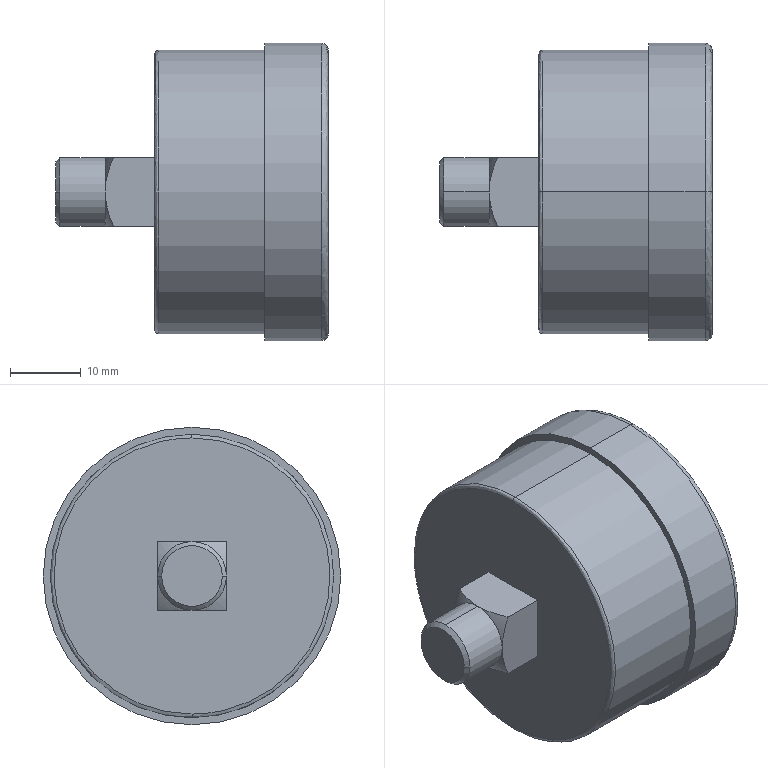Part | SolidWorks | features BaseBody 1 | 1 solid | 27 faces | box 38.5 x 42 x 42 mm | volume 31963 mm3 | plane 9 | cylinder 8 | spline 4 | torus 4 | cone 2 | commonest cylinder face diameters 9.728 x2 37.8 x2 40 x2 42 x2
STEP:
#1=CARTESIAN_POINT('',(0.5,0.,20.));
#2=VERTEX_POINT('',#1);
#3=CARTESIAN_POINT('',(0.5,0.,-20.));
#4=VERTEX_POINT('',#3);
#5=CARTESIAN_POINT('',(0.5,0.,0.));
#6=DIRECTION('',(1.,0.,0.));
#7=DIRECTION('',(0.,0.,1.));
#8=AXIS2_PLACEMENT_3D('',#5,#6,#7);
#9=CIRCLE('',#8,20.);
#10=EDGE_CURVE('',#2,#4,#9,.T.);
#11=ORIENTED_EDGE('',*,*,#10,.F.);
#12=CARTESIAN_POINT('',(0.,0.,19.5));
#13=VERTEX_POINT('',#12);
#14=CARTESIAN_POINT('',(0.5,0.,19.5));
#15=DIRECTION('',(0.,-1.,0.));
#16=DIRECTION('',(0.,0.,1.));
#17=AXIS2_PLACEMENT_3D('',#14,#15,#16);
#18=CIRCLE('',#17,0.5);
#19=EDGE_CURVE('',#2,#13,#18,.T.);
#20=ORIENTED_EDGE('',*,*,#19,.T.);
#21=CARTESIAN_POINT('',(0.,0.,-19.5));
#22=VERTEX_POINT('',#21);
#23=CARTESIAN_POINT('',(0.,0.,19.5));
#24=CARTESIAN_POINT('',(0.,-39.,19.5));
#25=CARTESIAN_POINT('',(0.,-39.,-19.5));
#26=CARTESIAN_POINT('',(0.,0.,-19.5));
#27=(BOUNDED_CURVE()B_SPLINE_CURVE(3,(#23,#24,#25,#26),.UNSPECIFIED.,.F.,.F.)B_SPLINE_CURVE_WITH_KNOTS((4,4),(0.5,1.),.UNSPECIFIED.)CURVE()GEOMETRIC_REPRESENTATION_ITEM()RATIONAL_B_SPLINE_CURVE((1.,0.3333,0.3333,1.))REPRESENTATION_ITEM(''));
#28=EDGE_CURVE('',#13,#22,#27,.T.);
#29=ORIENTED_EDGE('',*,*,#28,.T.);
#30=CARTESIAN_POINT('',(0.5,0.,-19.5));
#31=DIRECTION('',(0.,1.,0.));
#32=DIRECTION('',(0.,0.,-1.));
#33=AXIS2_PLACEMENT_3D('',#30,#31,#32);
#34=CIRCLE('',#33,0.5);
#35=EDGE_CURVE('',#4,#22,#34,.T.);
#36=ORIENTED_EDGE('',*,*,#35,.F.);
#37=EDGE_LOOP('',(#11,#20,#29,#36));
#38=FACE_OUTER_BOUND('',#37,.T.);
#39=CARTESIAN_POINT('',(0.5,0.,20.));
#40=CARTESIAN_POINT('',(0.5,-40.,20.));
#41=CARTESIAN_POINT('',(0.5,-40.,-20.));
#42=CARTESIAN_POINT('',(0.5,0.,-20.));
#43=CARTESIAN_POINT('',(0.2071,0.,20.));
#44=CARTESIAN_POINT('',(0.2071,-40.,20.));
#45=CARTESIAN_POINT('',(0.2071,-40.,-20.));
#46=CARTESIAN_POINT('',(0.2071,0.,-20.));
#47=CARTESIAN_POINT('',(0.,0.,19.793));
#48=CARTESIAN_POINT('',(0.,-39.586,19.793));
#49=CARTESIAN_POINT('',(0.,-39.586,-19.793));
#50=CARTESIAN_POINT('',(0.,0.,-19.793));
#51=CARTESIAN_POINT('',(0.,0.,19.5));
#52=CARTESIAN_POINT('',(0.,-39.,19.5));
#53=CARTESIAN_POINT('',(0.,-39.,-19.5));
#54=CARTESIAN_POINT('',(0.,0.,-19.5));
#55=(BOUNDED_SURFACE()B_SPLINE_SURFACE(3,3,((#39,#40,#41,#42),(#43,#44,#45,#46),(#47,#48,#49,#50),(#51,#52,#53,#54)),.UNSPECIFIED.,.F.,.F.,.F.)B_SPLINE_SURFACE_WITH_KNOTS((4,4),(4,4),(0.,1.),(0.,1.),.UNSPECIFIED.)GEOMETRIC_REPRESENTATION_ITEM()RATIONAL_B_SPLINE_SURFACE(((1.,0.3333,0.3333,1.),(0.8047,0.2682,0.2682,0.8047),(0.8047,0.2682,0.2682,0.8047),(1.,0.3333,0.3333,1.)))REPRESENTATION_ITEM('')SURFACE());
#56=ADVANCED_FACE('',(#38),#55,.T.);
#57=CARTESIAN_POINT('',(24.5,0.,-20.));
#58=VERTEX_POINT('',#57);
#59=CARTESIAN_POINT('',(24.5,0.,20.));
#60=VERTEX_POINT('',#59);
#61=CARTESIAN_POINT('',(24.5,0.,-20.));
#62=CARTESIAN_POINT('',(24.5,-40.,-20.));
#63=CARTESIAN_POINT('',(24.5,-40.,20.));
#64=CARTESIAN_POINT('',(24.5,0.,20.));
#65=(BOUNDED_CURVE()B_SPLINE_CURVE(3,(#61,#62,#63,#64),.UNSPECIFIED.,.F.,.T.)B_SPLINE_CURVE_WITH_KNOTS((4,4),(0.,0.5),.UNSPECIFIED.)CURVE()GEOMETRIC_REPRESENTATION_ITEM()RATIONAL_B_SPLINE_CURVE((1.,0.3333,0.3333,1.))REPRESENTATION_ITEM(''));
#66=EDGE_CURVE('',#58,#60,#65,.T.);
#67=ORIENTED_EDGE('',*,*,#66,.T.);
#68=CARTESIAN_POINT('',(23.5,0.,21.));
#69=VERTEX_POINT('',#68);
#70=CARTESIAN_POINT('',(23.5,0.,20.));
#71=DIRECTION('',(0.,-1.,0.));
#72=DIRECTION('',(0.,0.,1.));
#73=AXIS2_PLACEMENT_3D('',#70,#71,#72);
#74=CIRCLE('',#73,1.);
#75=EDGE_CURVE('',#60,#69,#74,.T.);
#76=ORIENTED_EDGE('',*,*,#75,.T.);
#77=CARTESIAN_POINT('',(23.5,0.,-21.));
#78=VERTEX_POINT('',#77);
#79=CARTESIAN_POINT('',(23.5,0.,0.));
#80=DIRECTION('',(-1.,0.,0.));
#81=DIRECTION('',(0.,0.,1.));
#82=AXIS2_PLACEMENT_3D('',#79,#80,#81);
#83=CIRCLE('',#82,21.);
#84=EDGE_CURVE('',#78,#69,#83,.T.);
#85=ORIENTED_EDGE('',*,*,#84,.F.);
#86=CARTESIAN_POINT('',(23.5,0.,-20.));
#87=DIRECTION('',(0.,1.,0.));
#88=DIRECTION('',(0.,0.,-1.));
#89=AXIS2_PLACEMENT_3D('',#86,#87,#88);
#90=CIRCLE('',#89,1.);
#91=EDGE_CURVE('',#58,#78,#90,.T.);
#92=ORIENTED_EDGE('',*,*,#91,.F.);
#93=EDGE_LOOP('',(#67,#76,#85,#92));
#94=FACE_OUTER_BOUND('',#93,.T.);
#95=CARTESIAN_POINT('',(24.5,0.,20.));
#96=CARTESIAN_POINT('',(24.5,-40.,20.));
#97=CARTESIAN_POINT('',(24.5,-40.,-20.));
#98=CARTESIAN_POINT('',(24.5,0.,-20.));
#99=CARTESIAN_POINT('',(24.5,0.,20.586));
#100=CARTESIAN_POINT('',(24.5,-41.172,20.586));
#101=CARTESIAN_POINT('',(24.5,-41.172,-20.586));
#102=CARTESIAN_POINT('',(24.5,0.,-20.586));
#103=CARTESIAN_POINT('',(24.086,0.,21.));
#104=CARTESIAN_POINT('',(24.086,-42.,21.));
#105=CARTESIAN_POINT('',(24.086,-42.,-21.));
#106=CARTESIAN_POINT('',(24.086,0.,-21.));
#107=CARTESIAN_POINT('',(23.5,0.,21.));
#108=CARTESIAN_POINT('',(23.5,-42.,21.));
#109=CARTESIAN_POINT('',(23.5,-42.,-21.));
#110=CARTESIAN_POINT('',(23.5,0.,-21.));
#111=(BOUNDED_SURFACE()B_SPLINE_SURFACE(3,3,((#95,#96,#97,#98),(#99,#100,#101,#102),(#103,#104,#105,#106),(#107,#108,#109,#110)),.UNSPECIFIED.,.F.,.F.,.F.)B_SPLINE_SURFACE_WITH_KNOTS((4,4),(4,4),(0.,1.),(0.,1.),.UNSPECIFIED.)GEOMETRIC_REPRESENTATION_ITEM()RATIONAL_B_SPLINE_SURFACE(((1.,0.3333,0.3333,1.),(0.8047,0.2682,0.2682,0.8047),(0.8047,0.2682,0.2682,0.8047),(1.,0.3333,0.3333,1.)))REPRESENTATION_ITEM('')SURFACE());
#112=ADVANCED_FACE('',(#94),#111,.T.);
#113=CARTESIAN_POINT('',(15.5,0.,20.));
#114=VERTEX_POINT('',#113);
#115=CARTESIAN_POINT('',(15.5,0.,-20.));
#116=VERTEX_POINT('',#115);
#117=CARTESIAN_POINT('',(15.5,0.,0.));
#118=DIRECTION('',(-1.,0.,0.));
#119=DIRECTION('',(0.,0.,1.));
#120=AXIS2_PLACEMENT_3D('',#117,#118,#119);
#121=CIRCLE('',#120,20.);
#122=EDGE_CURVE('',#114,#116,#121,.T.);
#123=ORIENTED_EDGE('',*,*,#122,.T.);
#124=CARTESIAN_POINT('',(23.5,0.,-20.));
#125=DIRECTION('',(-1.,0.,0.));
#126=VECTOR('',#125,1000.);
#127=LINE('',#124,#126);
#128=EDGE_CURVE('',#116,#4,#127,.T.);
#129=ORIENTED_EDGE('',*,*,#128,.T.);
#130=CARTESIAN_POINT('',(0.5,0.,0.));
#131=DIRECTION('',(1.,0.,0.));
#132=DIRECTION('',(0.,0.,1.));
#133=AXIS2_PLACEMENT_3D('',#130,#131,#132);
#134=CIRCLE('',#133,20.);
#135=EDGE_CURVE('',#4,#2,#134,.T.);
#136=ORIENTED_EDGE('',*,*,#135,.T.);
#137=CARTESIAN_POINT('',(23.5,0.,20.));
#138=DIRECTION('',(-1.,0.,0.));
#139=VECTOR('',#138,1000.);
#140=LINE('',#137,#139);
#141=EDGE_CURVE('',#114,#2,#140,.T.);
#142=ORIENTED_EDGE('',*,*,#141,.F.);
#143=EDGE_LOOP('',(#123,#129,#136,#142));
#144=FACE_OUTER_BOUND('',#143,.T.);
#145=CARTESIAN_POINT('',(23.5,0.,0.));
#146=DIRECTION('',(-1.,0.,0.));
#147=DIRECTION('',(0.,0.,1.));
#148=AXIS2_PLACEMENT_3D('',#145,#146,#147);
#149=CYLINDRICAL_SURFACE('',#148,20.);
#150=ADVANCED_FACE('',(#144),#149,.T.);
#151=CARTESIAN_POINT('',(23.5,0.,0.));
#152=DIRECTION('',(-1.,0.,0.));
#153=DIRECTION('',(0.,0.,1.));
#154=AXIS2_PLACEMENT_3D('',#151,#152,#153);
#155=CIRCLE('',#154,21.);
#156=EDGE_CURVE('',#69,#78,#155,.T.);
#157=ORIENTED_EDGE('',*,*,#156,.T.);
#158=CARTESIAN_POINT('',(15.5,0.,-21.));
#159=VERTEX_POINT('',#158);
#160=CARTESIAN_POINT('',(23.5,0.,-21.));
#161=DIRECTION('',(-1.,0.,0.));
#162=VECTOR('',#161,1000.);
#163=LINE('',#160,#162);
#164=EDGE_CURVE('',#78,#159,#163,.T.);
#165=ORIENTED_EDGE('',*,*,#164,.T.);
#166=CARTESIAN_POINT('',(15.5,0.,21.));
#167=VERTEX_POINT('',#166);
#168=CARTESIAN_POINT('',(15.5,0.,0.));
#169=DIRECTION('',(1.,0.,0.));
#170=DIRECTION('',(0.,0.,1.));
#171=AXIS2_PLACEMENT_3D('',#168,#169,#170);
#172=CIRCLE('',#171,21.);
#173=EDGE_CURVE('',#159,#167,#172,.T.);
#174=ORIENTED_EDGE('',*,*,#173,.T.);
#175=CARTESIAN_POINT('',(23.5,0.,21.));
#176=DIRECTION('',(-1.,0.,0.));
#177=VECTOR('',#176,1000.);
#178=LINE('',#175,#177);
#179=EDGE_CURVE('',#69,#167,#178,.T.);
#180=ORIENTED_EDGE('',*,*,#179,.F.);
#181=EDGE_LOOP('',(#157,#165,#174,#180));
#182=FACE_OUTER_BOUND('',#181,.T.);
#183=CARTESIAN_POINT('',(23.5,0.,0.));
#184=DIRECTION('',(-1.,0.,0.));
#185=DIRECTION('',(0.,0.,1.));
#186=AXIS2_PLACEMENT_3D('',#183,#184,#185);
#187=CYLINDRICAL_SURFACE('',#186,21.);
#188=ADVANCED_FACE('',(#182),#187,.T.);
#189=CARTESIAN_POINT('',(-7.,0.,-4.864));
#190=VERTEX_POINT('',#189);
#191=CARTESIAN_POINT('',(-7.,4.864,0.));
#192=VERTEX_POINT('',#191);
#193=CARTESIAN_POINT('',(-7.,0.,0.));
#194=DIRECTION('',(1.,0.,0.));
#195=DIRECTION('',(0.,0.,-1.));
#196=AXIS2_PLACEMENT_3D('',#193,#194,#195);
#197=CIRCLE('',#196,4.864);
#198=EDGE_CURVE('',#190,#192,#197,.T.);
#199=ORIENTED_EDGE('',*,*,#198,.F.);
#200=CARTESIAN_POINT('',(-13.419,0.,-4.864));
#201=VERTEX_POINT('',#200);
#202=CARTESIAN_POINT('',(23.5,0.,-4.864));
#203=DIRECTION('',(-1.,0.,0.));
#204=VECTOR('',#203,1000.);
#205=LINE('',#202,#204);
#206=EDGE_CURVE('',#190,#201,#205,.T.);
#207=ORIENTED_EDGE('',*,*,#206,.T.);
#208=CARTESIAN_POINT('',(-13.419,4.864,0.));
#209=VERTEX_POINT('',#208);
#210=CARTESIAN_POINT('',(-13.419,0.,0.));
#211=DIRECTION('',(1.,0.,0.));
#212=DIRECTION('',(0.,0.,1.));
#213=AXIS2_PLACEMENT_3D('',#210,#211,#212);
#214=CIRCLE('',#213,4.864);
#215=EDGE_CURVE('',#201,#209,#214,.T.);
#216=ORIENTED_EDGE('',*,*,#215,.T.);
#217=CARTESIAN_POINT('',(-13.419,0.,4.864));
#218=VERTEX_POINT('',#217);
#219=CARTESIAN_POINT('',(-13.419,0.,0.));
#220=DIRECTION('',(1.,0.,0.));
#221=DIRECTION('',(0.,0.,1.));
#222=AXIS2_PLACEMENT_3D('',#219,#220,#221);
#223=CIRCLE('',#222,4.864);
#224=EDGE_CURVE('',#209,#218,#223,.T.);
#225=ORIENTED_EDGE('',*,*,#224,.T.);
#226=CARTESIAN_POINT('',(-7.,0.,4.864));
#227=VERTEX_POINT('',#226);
#228=CARTESIAN_POINT('',(23.5,0.,4.864));
#229=DIRECTION('',(-1.,0.,0.));
#230=VECTOR('',#229,1000.);
#231=LINE('',#228,#230);
#232=EDGE_CURVE('',#227,#218,#231,.T.);
#233=ORIENTED_EDGE('',*,*,#232,.F.);
#234=CARTESIAN_POINT('',(-7.,0.,0.));
#235=DIRECTION('',(1.,0.,0.));
#236=DIRECTION('',(0.,1.,0.));
#237=AXIS2_PLACEMENT_3D('',#234,#235,#236);
#238=CIRCLE('',#237,4.864);
#239=EDGE_CURVE('',#192,#227,#238,.T.);
#240=ORIENTED_EDGE('',*,*,#239,.F.);
#241=EDGE_LOOP('',(#199,#207,#216,#225,#233,#240));
#242=FACE_OUTER_BOUND('',#241,.T.);
#243=CARTESIAN_POINT('',(23.5,0.,0.));
#244=DIRECTION('',(-1.,0.,0.));
#245=DIRECTION('',(0.,0.,1.));
#246=AXIS2_PLACEMENT_3D('',#243,#244,#245);
#247=CYLINDRICAL_SURFACE('',#246,4.864);
#248=ADVANCED_FACE('',(#242),#247,.T.);
#249=CARTESIAN_POINT('',(24.5,0.,18.9));
#250=VERTEX_POINT('',#249);
#251=CARTESIAN_POINT('',(24.5,0.,-18.9));
#252=VERTEX_POINT('',#251);
#253=CARTESIAN_POINT('',(24.5,0.,0.));
#254=DIRECTION('',(1.,0.,0.));
#255=DIRECTION('',(0.,0.,1.));
#256=AXIS2_PLACEMENT_3D('',#253,#254,#255);
#257=CIRCLE('',#256,18.9);
#258=EDGE_CURVE('',#250,#252,#257,.T.);
#259=ORIENTED_EDGE('',*,*,#258,.T.);
#260=CARTESIAN_POINT('',(23.5,0.,-18.9));
#261=VERTEX_POINT('',#260);
#262=CARTESIAN_POINT('',(23.5,0.,-18.9));
#263=DIRECTION('',(-1.,0.,0.));
#264=VECTOR('',#263,1000.);
#265=LINE('',#262,#264);
#266=EDGE_CURVE('',#252,#261,#265,.T.);
#267=ORIENTED_EDGE('',*,*,#266,.T.);
#268=CARTESIAN_POINT('',(23.5,0.,18.9));
#269=VERTEX_POINT('',#268);
#270=CARTESIAN_POINT('',(23.5,0.,0.));
#271=DIRECTION('',(1.,0.,0.));
#272=DIRECTION('',(0.,0.,1.));
#273=AXIS2_PLACEMENT_3D('',#270,#271,#272);
#274=CIRCLE('',#273,18.9);
#275=EDGE_CURVE('',#269,#261,#274,.T.);
#276=ORIENTED_EDGE('',*,*,#275,.F.);
#277=CARTESIAN_POINT('',(23.5,0.,18.9));
#278=DIRECTION('',(-1.,0.,0.));
#279=VECTOR('',#278,1000.);
#280=LINE('',#277,#279);
#281=EDGE_CURVE('',#250,#269,#280,.T.);
#282=ORIENTED_EDGE('',*,*,#281,.F.);
#283=EDGE_LOOP('',(#259,#267,#276,#282));
#284=FACE_OUTER_BOUND('',#283,.T.);
#285=CARTESIAN_POINT('',(23.5,0.,0.));
#286=DIRECTION('',(-1.,0.,0.));
#287=DIRECTION('',(0.,0.,1.));
#288=AXIS2_PLACEMENT_3D('',#285,#286,#287);
#289=CYLINDRICAL_SURFACE('',#288,18.9);
#290=ADVANCED_FACE('',(#284),#289,.F.);
#291=CARTESIAN_POINT('',(-14.,4.283,0.));
#292=VERTEX_POINT('',#291);
#293=CARTESIAN_POINT('',(-14.,-4.283,0.));
#294=VERTEX_POINT('',#293);
#295=CARTESIAN_POINT('',(-14.,0.,0.));
#296=DIRECTION('',(1.,0.,0.));
#297=DIRECTION('',(0.,1.,0.));
#298=AXIS2_PLACEMENT_3D('',#295,#296,#297);
#299=CIRCLE('',#298,4.283);
#300=EDGE_CURVE('',#292,#294,#299,.T.);
#301=ORIENTED_EDGE('',*,*,#300,.T.);
#302=CARTESIAN_POINT('',(-13.419,-4.864,0.));
#303=VERTEX_POINT('',#302);
#304=CARTESIAN_POINT('',(-13.419,-4.864,0.));
#305=DIRECTION('',(0.7071,-0.7071,0.));
#306=VECTOR('',#305,1000.);
#307=LINE('',#304,#306);
#308=EDGE_CURVE('',#294,#303,#307,.T.);
#309=ORIENTED_EDGE('',*,*,#308,.T.);
#310=CARTESIAN_POINT('',(-13.419,0.,0.));
#311=DIRECTION('',(1.,0.,0.));
#312=DIRECTION('',(0.,0.,1.));
#313=AXIS2_PLACEMENT_3D('',#310,#311,#312);
#314=CIRCLE('',#313,4.864);
#315=EDGE_CURVE('',#218,#303,#314,.T.);
#316=ORIENTED_EDGE('',*,*,#315,.F.);
#317=ORIENTED_EDGE('',*,*,#224,.F.);
#318=CARTESIAN_POINT('',(-13.419,4.864,0.));
#319=DIRECTION('',(0.7071,0.7071,0.));
#320=VECTOR('',#319,1000.);
#321=LINE('',#318,#320);
#322=EDGE_CURVE('',#292,#209,#321,.T.);
#323=ORIENTED_EDGE('',*,*,#322,.F.);
#324=EDGE_LOOP('',(#301,#309,#316,#317,#323));
#325=FACE_OUTER_BOUND('',#324,.T.);
#326=CARTESIAN_POINT('',(-13.419,0.,0.));
#327=DIRECTION('',(1.,0.,0.));
#328=DIRECTION('',(0.,1.,0.));
#329=AXIS2_PLACEMENT_3D('',#326,#327,#328);
#330=CONICAL_SURFACE('',#329,4.864,0.7854);
#331=ADVANCED_FACE('',(#325),#330,.T.);
#332=ORIENTED_EDGE('',*,*,#128,.F.);
#333=CARTESIAN_POINT('',(15.5,0.,0.));
#334=DIRECTION('',(-1.,0.,0.));
#335=DIRECTION('',(0.,0.,1.));
#336=AXIS2_PLACEMENT_3D('',#333,#334,#335);
#337=CIRCLE('',#336,20.);
#338=EDGE_CURVE('',#116,#114,#337,.T.);
#339=ORIENTED_EDGE('',*,*,#338,.T.);
#340=ORIENTED_EDGE('',*,*,#141,.T.);
#341=ORIENTED_EDGE('',*,*,#10,.T.);
#342=EDGE_LOOP('',(#332,#339,#340,#341));
#343=FACE_OUTER_BOUND('',#342,.T.);
#344=CARTESIAN_POINT('',(23.5,0.,0.));
#345=DIRECTION('',(-1.,0.,0.));
#346=DIRECTION('',(0.,0.,1.));
#347=AXIS2_PLACEMENT_3D('',#344,#345,#346);
#348=CYLINDRICAL_SURFACE('',#347,20.);
#349=ADVANCED_FACE('',(#343),#348,.T.);
#350=ORIENTED_EDGE('',*,*,#19,.F.);
#351=ORIENTED_EDGE('',*,*,#135,.F.);
#352=ORIENTED_EDGE('',*,*,#35,.T.);
#353=CARTESIAN_POINT('',(0.,0.,-19.5));
#354=CARTESIAN_POINT('',(0.,39.,-19.5));
#355=CARTESIAN_POINT('',(0.,39.,19.5));
#356=CARTESIAN_POINT('',(0.,0.,19.5));
#357=(BOUNDED_CURVE()B_SPLINE_CURVE(3,(#353,#354,#355,#356),.UNSPECIFIED.,.F.,.F.)B_SPLINE_CURVE_WITH_KNOTS((4,4),(0.,0.5),.UNSPECIFIED.)CURVE()GEOMETRIC_REPRESENTATION_ITEM()RATIONAL_B_SPLINE_CURVE((1.,0.3333,0.3333,1.))REPRESENTATION_ITEM(''));
#358=EDGE_CURVE('',#22,#13,#357,.T.);
#359=ORIENTED_EDGE('',*,*,#358,.T.);
#360=EDGE_LOOP('',(#350,#351,#352,#359));
#361=FACE_OUTER_BOUND('',#360,.T.);
#362=CARTESIAN_POINT('',(0.5,0.,-20.));
#363=CARTESIAN_POINT('',(0.5,40.,-20.));
#364=CARTESIAN_POINT('',(0.5,40.,20.));
#365=CARTESIAN_POINT('',(0.5,0.,20.));
#366=CARTESIAN_POINT('',(0.2071,0.,-20.));
#367=CARTESIAN_POINT('',(0.2071,40.,-20.));
#368=CARTESIAN_POINT('',(0.2071,40.,20.));
#369=CARTESIAN_POINT('',(0.2071,0.,20.));
#370=CARTESIAN_POINT('',(0.,0.,-19.793));
#371=CARTESIAN_POINT('',(0.,39.586,-19.793));
#372=CARTESIAN_POINT('',(0.,39.586,19.793));
#373=CARTESIAN_POINT('',(0.,0.,19.793));
#374=CARTESIAN_POINT('',(0.,0.,-19.5));
#375=CARTESIAN_POINT('',(0.,39.,-19.5));
#376=CARTESIAN_POINT('',(0.,39.,19.5));
#377=CARTESIAN_POINT('',(0.,0.,19.5));
#378=(BOUNDED_SURFACE()B_SPLINE_SURFACE(3,3,((#362,#363,#364,#365),(#366,#367,#368,#369),(#370,#371,#372,#373),(#374,#375,#376,#377)),.UNSPECIFIED.,.F.,.F.,.F.)B_SPLINE_SURFACE_WITH_KNOTS((4,4),(4,4),(0.,1.),(0.,1.),.UNSPECIFIED.)GEOMETRIC_REPRESENTATION_ITEM()RATIONAL_B_SPLINE_SURFACE(((1.,0.3333,0.3333,1.),(0.8047,0.2682,0.2682,0.8047),(0.8047,0.2682,0.2682,0.8047),(1.,0.3333,0.3333,1.)))REPRESENTATION_ITEM('')SURFACE());
#379=ADVANCED_FACE('',(#361),#378,.T.);
#380=ORIENTED_EDGE('',*,*,#122,.F.);
#381=ORIENTED_EDGE('',*,*,#338,.F.);
#382=EDGE_LOOP('',(#380,#381));
#383=FACE_BOUND('',#382,.T.);
#384=CARTESIAN_POINT('',(15.5,0.,0.));
#385=DIRECTION('',(1.,0.,0.));
#386=DIRECTION('',(0.,0.,1.));
#387=AXIS2_PLACEMENT_3D('',#384,#385,#386);
#388=CIRCLE('',#387,21.);
#389=EDGE_CURVE('',#167,#159,#388,.T.);
#390=ORIENTED_EDGE('',*,*,#389,.F.);
#391=ORIENTED_EDGE('',*,*,#173,.F.);
#392=EDGE_LOOP('',(#390,#391));
#393=FACE_OUTER_BOUND('',#392,.T.);
#394=CARTESIAN_POINT('',(15.5,20.,0.));
#395=DIRECTION('',(1.,0.,0.));
#396=DIRECTION('',(0.,0.,-1.));
#397=AXIS2_PLACEMENT_3D('',#394,#395,#396);
#398=PLANE('',#397);
#399=ADVANCED_FACE('',(#383,#393),#398,.F.);
#400=CARTESIAN_POINT('',(0.,-4.864,4.864));
#401=VERTEX_POINT('',#400);
#402=CARTESIAN_POINT('',(0.,4.864,4.864));
#403=VERTEX_POINT('',#402);
#404=CARTESIAN_POINT('',(0.,4.864,4.864));
#405=DIRECTION('',(0.,1.,0.));
#406=VECTOR('',#405,1000.);
#407=LINE('',#404,#406);
#408=EDGE_CURVE('',#401,#403,#407,.T.);
#409=ORIENTED_EDGE('',*,*,#408,.F.);
#410=CARTESIAN_POINT('',(0.,-4.864,-4.864));
#411=VERTEX_POINT('',#410);
#412=CARTESIAN_POINT('',(0.,-4.864,0.));
#413=DIRECTION('',(0.,0.,1.));
#414=VECTOR('',#413,1000.);
#415=LINE('',#412,#414);
#416=EDGE_CURVE('',#411,#401,#415,.T.);
#417=ORIENTED_EDGE('',*,*,#416,.F.);
#418=CARTESIAN_POINT('',(0.,4.864,-4.864));
#419=VERTEX_POINT('',#418);
#420=CARTESIAN_POINT('',(0.,4.864,-4.864));
#421=DIRECTION('',(0.,-1.,0.));
#422=VECTOR('',#421,1000.);
#423=LINE('',#420,#422);
#424=EDGE_CURVE('',#419,#411,#423,.T.);
#425=ORIENTED_EDGE('',*,*,#424,.F.);
#426=CARTESIAN_POINT('',(0.,4.864,0.));
#427=DIRECTION('',(0.,0.,-1.));
#428=VECTOR('',#427,1000.);
#429=LINE('',#426,#428);
#430=EDGE_CURVE('',#403,#419,#429,.T.);
#431=ORIENTED_EDGE('',*,*,#430,.F.);
#432=EDGE_LOOP('',(#409,#417,#425,#431));
#433=FACE_BOUND('',#432,.T.);
#434=ORIENTED_EDGE('',*,*,#358,.F.);
#435=ORIENTED_EDGE('',*,*,#28,.F.);
#436=EDGE_LOOP('',(#434,#435));
#437=FACE_OUTER_BOUND('',#436,.T.);
#438=CARTESIAN_POINT('',(0.,4.864,0.));
#439=DIRECTION('',(1.,0.,0.));
#440=DIRECTION('',(0.,0.,-1.));
#441=AXIS2_PLACEMENT_3D('',#438,#439,#440);
#442=PLANE('',#441);
#443=ADVANCED_FACE('',(#433,#437),#442,.F.);
#444=ORIENTED_EDGE('',*,*,#164,.F.);
#445=ORIENTED_EDGE('',*,*,#84,.T.);
#446=ORIENTED_EDGE('',*,*,#179,.T.);
#447=ORIENTED_EDGE('',*,*,#389,.T.);
#448=EDGE_LOOP('',(#444,#445,#446,#447));
#449=FACE_OUTER_BOUND('',#448,.T.);
#450=CARTESIAN_POINT('',(23.5,0.,0.));
#451=DIRECTION('',(-1.,0.,0.));
#452=DIRECTION('',(0.,0.,1.));
#453=AXIS2_PLACEMENT_3D('',#450,#451,#452);
#454=CYLINDRICAL_SURFACE('',#453,21.);
#455=ADVANCED_FACE('',(#449),#454,.T.);
#456=CARTESIAN_POINT('',(-5.815,4.864,-4.864));
#457=VERTEX_POINT('',#456);
#458=CARTESIAN_POINT('',(-19.25,4.864,-4.864));
#459=DIRECTION('',(-1.,0.,0.));
#460=VECTOR('',#459,1000.);
#461=LINE('',#458,#460);
#462=EDGE_CURVE('',#419,#457,#461,.T.);
#463=ORIENTED_EDGE('',*,*,#462,.T.);
#464=CARTESIAN_POINT('',(-5.815,4.864,-4.864));
#465=CARTESIAN_POINT('',(-6.176,4.864,-4.1));
#466=CARTESIAN_POINT('',(-6.469,4.864,-3.315));
#467=CARTESIAN_POINT('',(-6.779,4.864,-2.099));
#468=CARTESIAN_POINT('',(-6.861,4.864,-1.687));
#469=CARTESIAN_POINT('',(-6.971,4.864,-0.8465));
#470=CARTESIAN_POINT('',(-7.,4.864,-0.424));
#471=CARTESIAN_POINT('',(-7.,4.864,0.));
#472=B_SPLINE_CURVE_WITH_KNOTS('',3,(#464,#465,#466,#467,#468,#469,#470,#471),.UNSPECIFIED.,.F.,.F.,(4,2,2,4),(0.,0.002508,0.003762,0.005016),.UNSPECIFIED.);
#473=EDGE_CURVE('',#457,#192,#472,.T.);
#474=ORIENTED_EDGE('',*,*,#473,.T.);
#475=CARTESIAN_POINT('',(-5.815,4.864,4.864));
#476=VERTEX_POINT('',#475);
#477=CARTESIAN_POINT('',(-7.,4.864,0.));
#478=CARTESIAN_POINT('',(-7.,4.864,0.8482));
#479=CARTESIAN_POINT('',(-6.886,4.864,1.677));
#480=CARTESIAN_POINT('',(-6.577,4.864,2.896));
#481=CARTESIAN_POINT('',(-6.451,4.864,3.3));
#482=CARTESIAN_POINT('',(-6.16,4.864,4.093));
#483=CARTESIAN_POINT('',(-5.996,4.864,4.482));
#484=CARTESIAN_POINT('',(-5.815,4.864,4.864));
#485=B_SPLINE_CURVE_WITH_KNOTS('',3,(#477,#478,#479,#480,#481,#482,#483,#484),.UNSPECIFIED.,.F.,.F.,(4,2,2,4),(0.,0.002508,0.003762,0.005015),.UNSPECIFIED.);
#486=EDGE_CURVE('',#192,#476,#485,.T.);
#487=ORIENTED_EDGE('',*,*,#486,.T.);
#488=CARTESIAN_POINT('',(-19.25,4.864,4.864));
#489=DIRECTION('',(1.,0.,0.));
#490=VECTOR('',#489,1000.);
#491=LINE('',#488,#490);
#492=EDGE_CURVE('',#476,#403,#491,.T.);
#493=ORIENTED_EDGE('',*,*,#492,.T.);
#494=ORIENTED_EDGE('',*,*,#430,.T.);
#495=EDGE_LOOP('',(#463,#474,#487,#493,#494));
#496=FACE_OUTER_BOUND('',#495,.T.);
#497=CARTESIAN_POINT('',(-19.25,4.864,-4.864));
#498=DIRECTION('',(0.,1.,0.));
#499=DIRECTION('',(0.,0.,1.));
#500=AXIS2_PLACEMENT_3D('',#497,#498,#499);
#501=PLANE('',#500);
#502=ADVANCED_FACE('',(#496),#501,.T.);
#503=ORIENTED_EDGE('',*,*,#492,.F.);
#504=CARTESIAN_POINT('',(-5.815,4.864,4.864));
#505=CARTESIAN_POINT('',(-6.176,4.1,4.864));
#506=CARTESIAN_POINT('',(-6.469,3.315,4.864));
#507=CARTESIAN_POINT('',(-6.779,2.099,4.864));
#508=CARTESIAN_POINT('',(-6.861,1.687,4.864));
#509=CARTESIAN_POINT('',(-6.971,0.8465,4.864));
#510=CARTESIAN_POINT('',(-7.,0.424,4.864));
#511=CARTESIAN_POINT('',(-7.,0.,4.864));
#512=B_SPLINE_CURVE_WITH_KNOTS('',3,(#504,#505,#506,#507,#508,#509,#510,#511),.UNSPECIFIED.,.F.,.F.,(4,2,2,4),(0.,0.002508,0.003762,0.005016),.UNSPECIFIED.);
#513=EDGE_CURVE('',#476,#227,#512,.T.);
#514=ORIENTED_EDGE('',*,*,#513,.T.);
#515=CARTESIAN_POINT('',(-5.815,-4.864,4.864));
#516=VERTEX_POINT('',#515);
#517=CARTESIAN_POINT('',(-7.,0.,4.864));
#518=CARTESIAN_POINT('',(-7.,-0.8482,4.864));
#519=CARTESIAN_POINT('',(-6.886,-1.677,4.864));
#520=CARTESIAN_POINT('',(-6.577,-2.896,4.864));
#521=CARTESIAN_POINT('',(-6.451,-3.3,4.864));
#522=CARTESIAN_POINT('',(-6.16,-4.093,4.864));
#523=CARTESIAN_POINT('',(-5.996,-4.482,4.864));
#524=CARTESIAN_POINT('',(-5.815,-4.864,4.864));
#525=B_SPLINE_CURVE_WITH_KNOTS('',3,(#517,#518,#519,#520,#521,#522,#523,#524),.UNSPECIFIED.,.F.,.F.,(4,2,2,4),(0.,0.002508,0.003762,0.005015),.UNSPECIFIED.);
#526=EDGE_CURVE('',#227,#516,#525,.T.);
#527=ORIENTED_EDGE('',*,*,#526,.T.);
#528=CARTESIAN_POINT('',(-19.25,-4.864,4.864));
#529=DIRECTION('',(1.,0.,0.));
#530=VECTOR('',#529,1000.);
#531=LINE('',#528,#530);
#532=EDGE_CURVE('',#516,#401,#531,.T.);
#533=ORIENTED_EDGE('',*,*,#532,.T.);
#534=ORIENTED_EDGE('',*,*,#408,.T.);
#535=EDGE_LOOP('',(#503,#514,#527,#533,#534));
#536=FACE_OUTER_BOUND('',#535,.T.);
#537=CARTESIAN_POINT('',(-19.25,4.864,4.864));
#538=DIRECTION('',(0.,0.,1.));
#539=DIRECTION('',(1.,0.,0.));
#540=AXIS2_PLACEMENT_3D('',#537,#538,#539);
#541=PLANE('',#540);
#542=ADVANCED_FACE('',(#536),#541,.T.);
#543=ORIENTED_EDGE('',*,*,#532,.F.);
#544=CARTESIAN_POINT('',(-7.,-4.864,0.));
#545=VERTEX_POINT('',#544);
#546=CARTESIAN_POINT('',(-5.815,-4.864,4.864));
#547=CARTESIAN_POINT('',(-6.176,-4.864,4.1));
#548=CARTESIAN_POINT('',(-6.469,-4.864,3.315));
#549=CARTESIAN_POINT('',(-6.779,-4.864,2.099));
#550=CARTESIAN_POINT('',(-6.861,-4.864,1.687));
#551=CARTESIAN_POINT('',(-6.971,-4.864,0.8465));
#552=CARTESIAN_POINT('',(-7.,-4.864,0.424));
#553=CARTESIAN_POINT('',(-7.,-4.864,0.));
#554=B_SPLINE_CURVE_WITH_KNOTS('',3,(#546,#547,#548,#549,#550,#551,#552,#553),.UNSPECIFIED.,.F.,.F.,(4,2,2,4),(0.,0.002508,0.003762,0.005016),.UNSPECIFIED.);
#555=EDGE_CURVE('',#516,#545,#554,.T.);
#556=ORIENTED_EDGE('',*,*,#555,.T.);
#557=CARTESIAN_POINT('',(-5.815,-4.864,-4.864));
#558=VERTEX_POINT('',#557);
#559=CARTESIAN_POINT('',(-7.,-4.864,0.));
#560=CARTESIAN_POINT('',(-7.,-4.864,-0.8482));
#561=CARTESIAN_POINT('',(-6.886,-4.864,-1.677));
#562=CARTESIAN_POINT('',(-6.577,-4.864,-2.896));
#563=CARTESIAN_POINT('',(-6.451,-4.864,-3.3));
#564=CARTESIAN_POINT('',(-6.16,-4.864,-4.093));
#565=CARTESIAN_POINT('',(-5.996,-4.864,-4.482));
#566=CARTESIAN_POINT('',(-5.815,-4.864,-4.864));
#567=B_SPLINE_CURVE_WITH_KNOTS('',3,(#559,#560,#561,#562,#563,#564,#565,#566),.UNSPECIFIED.,.F.,.F.,(4,2,2,4),(0.,0.002508,0.003762,0.005015),.UNSPECIFIED.);
#568=EDGE_CURVE('',#545,#558,#567,.T.);
#569=ORIENTED_EDGE('',*,*,#568,.T.);
#570=CARTESIAN_POINT('',(-19.25,-4.864,-4.864));
#571=DIRECTION('',(1.,0.,0.));
#572=VECTOR('',#571,1000.);
#573=LINE('',#570,#572);
#574=EDGE_CURVE('',#558,#411,#573,.T.);
#575=ORIENTED_EDGE('',*,*,#574,.T.);
#576=ORIENTED_EDGE('',*,*,#416,.T.);
#577=EDGE_LOOP('',(#543,#556,#569,#575,#576));
#578=FACE_OUTER_BOUND('',#577,.T.);
#579=CARTESIAN_POINT('',(-19.25,-4.864,4.864));
#580=DIRECTION('',(0.,-1.,0.));
#581=DIRECTION('',(0.,0.,-1.));
#582=AXIS2_PLACEMENT_3D('',#579,#580,#581);
#583=PLANE('',#582);
#584=ADVANCED_FACE('',(#578),#583,.T.);
#585=ORIENTED_EDGE('',*,*,#574,.F.);
#586=CARTESIAN_POINT('',(-5.815,-4.864,-4.864));
#587=CARTESIAN_POINT('',(-6.176,-4.1,-4.864));
#588=CARTESIAN_POINT('',(-6.469,-3.315,-4.864));
#589=CARTESIAN_POINT('',(-6.779,-2.099,-4.864));
#590=CARTESIAN_POINT('',(-6.861,-1.687,-4.864));
#591=CARTESIAN_POINT('',(-6.971,-0.8465,-4.864));
#592=CARTESIAN_POINT('',(-7.,-0.424,-4.864));
#593=CARTESIAN_POINT('',(-7.,0.,-4.864));
#594=B_SPLINE_CURVE_WITH_KNOTS('',3,(#586,#587,#588,#589,#590,#591,#592,#593),.UNSPECIFIED.,.F.,.F.,(4,2,2,4),(0.,0.002508,0.003762,0.005016),.UNSPECIFIED.);
#595=EDGE_CURVE('',#558,#190,#594,.T.);
#596=ORIENTED_EDGE('',*,*,#595,.T.);
#597=CARTESIAN_POINT('',(-7.,0.,-4.864));
#598=CARTESIAN_POINT('',(-7.,0.8482,-4.864));
#599=CARTESIAN_POINT('',(-6.886,1.677,-4.864));
#600=CARTESIAN_POINT('',(-6.577,2.896,-4.864));
#601=CARTESIAN_POINT('',(-6.451,3.3,-4.864));
#602=CARTESIAN_POINT('',(-6.16,4.093,-4.864));
#603=CARTESIAN_POINT('',(-5.996,4.482,-4.864));
#604=CARTESIAN_POINT('',(-5.815,4.864,-4.864));
#605=B_SPLINE_CURVE_WITH_KNOTS('',3,(#597,#598,#599,#600,#601,#602,#603,#604),.UNSPECIFIED.,.F.,.F.,(4,2,2,4),(0.,0.002508,0.003762,0.005015),.UNSPECIFIED.);
#606=EDGE_CURVE('',#190,#457,#605,.T.);
#607=ORIENTED_EDGE('',*,*,#606,.T.);
#608=ORIENTED_EDGE('',*,*,#462,.F.);
#609=ORIENTED_EDGE('',*,*,#424,.T.);
#610=EDGE_LOOP('',(#585,#596,#607,#608,#609));
#611=FACE_OUTER_BOUND('',#610,.T.);
#612=CARTESIAN_POINT('',(-19.25,-4.864,-4.864));
#613=DIRECTION('',(0.,0.,-1.));
#614=DIRECTION('',(-1.,0.,0.));
#615=AXIS2_PLACEMENT_3D('',#612,#613,#614);
#616=PLANE('',#615);
#617=ADVANCED_FACE('',(#611),#616,.T.);
#618=ORIENTED_EDGE('',*,*,#75,.F.);
#619=CARTESIAN_POINT('',(24.5,0.,20.));
#620=CARTESIAN_POINT('',(24.5,40.,20.));
#621=CARTESIAN_POINT('',(24.5,40.,-20.));
#622=CARTESIAN_POINT('',(24.5,0.,-20.));
#623=(BOUNDED_CURVE()B_SPLINE_CURVE(3,(#619,#620,#621,#622),.UNSPECIFIED.,.F.,.F.)B_SPLINE_CURVE_WITH_KNOTS((4,4),(0.5,1.),.UNSPECIFIED.)CURVE()GEOMETRIC_REPRESENTATION_ITEM()RATIONAL_B_SPLINE_CURVE((1.,0.3333,0.3333,1.))REPRESENTATION_ITEM(''));
#624=EDGE_CURVE('',#60,#58,#623,.T.);
#625=ORIENTED_EDGE('',*,*,#624,.T.);
#626=ORIENTED_EDGE('',*,*,#91,.T.);
#627=ORIENTED_EDGE('',*,*,#156,.F.);
#628=EDGE_LOOP('',(#618,#625,#626,#627));
#629=FACE_OUTER_BOUND('',#628,.T.);
#630=CARTESIAN_POINT('',(24.5,0.,-20.));
#631=CARTESIAN_POINT('',(24.5,40.,-20.));
#632=CARTESIAN_POINT('',(24.5,40.,20.));
#633=CARTESIAN_POINT('',(24.5,0.,20.));
#634=CARTESIAN_POINT('',(24.5,0.,-20.586));
#635=CARTESIAN_POINT('',(24.5,41.172,-20.586));
#636=CARTESIAN_POINT('',(24.5,41.172,20.586));
#637=CARTESIAN_POINT('',(24.5,0.,20.586));
#638=CARTESIAN_POINT('',(24.086,0.,-21.));
#639=CARTESIAN_POINT('',(24.086,42.,-21.));
#640=CARTESIAN_POINT('',(24.086,42.,21.));
#641=CARTESIAN_POINT('',(24.086,0.,21.));
#642=CARTESIAN_POINT('',(23.5,0.,-21.));
#643=CARTESIAN_POINT('',(23.5,42.,-21.));
#644=CARTESIAN_POINT('',(23.5,42.,21.));
#645=CARTESIAN_POINT('',(23.5,0.,21.));
#646=(BOUNDED_SURFACE()B_SPLINE_SURFACE(3,3,((#630,#631,#632,#633),(#634,#635,#636,#637),(#638,#639,#640,#641),(#642,#643,#644,#645)),.UNSPECIFIED.,.F.,.F.,.F.)B_SPLINE_SURFACE_WITH_KNOTS((4,4),(4,4),(0.,1.),(0.,1.),.UNSPECIFIED.)GEOMETRIC_REPRESENTATION_ITEM()RATIONAL_B_SPLINE_SURFACE(((1.,0.3333,0.3333,1.),(0.8047,0.2682,0.2682,0.8047),(0.8047,0.2682,0.2682,0.8047),(1.,0.3333,0.3333,1.)))REPRESENTATION_ITEM('')SURFACE());
#647=ADVANCED_FACE('',(#629),#646,.T.);
#648=ORIENTED_EDGE('',*,*,#606,.F.);
#649=ORIENTED_EDGE('',*,*,#198,.T.);
#650=ORIENTED_EDGE('',*,*,#473,.F.);
#651=EDGE_LOOP('',(#648,#649,#650));
#652=FACE_OUTER_BOUND('',#651,.T.);
#653=CARTESIAN_POINT('',(10.801,0.,0.));
#654=DIRECTION('',(1.,0.,0.));
#655=DIRECTION('',(0.,1.,0.));
#656=AXIS2_PLACEMENT_3D('',#653,#654,#655);
#657=TOROIDAL_SURFACE('',#656,-4.254,20.);
#658=ADVANCED_FACE('',(#652),#657,.T.);
#659=ORIENTED_EDGE('',*,*,#486,.F.);
#660=ORIENTED_EDGE('',*,*,#239,.T.);
#661=ORIENTED_EDGE('',*,*,#513,.F.);
#662=EDGE_LOOP('',(#659,#660,#661));
#663=FACE_OUTER_BOUND('',#662,.T.);
#664=CARTESIAN_POINT('',(10.801,0.,0.));
#665=DIRECTION('',(1.,0.,0.));
#666=DIRECTION('',(0.,1.,0.));
#667=AXIS2_PLACEMENT_3D('',#664,#665,#666);
#668=TOROIDAL_SURFACE('',#667,-4.254,20.);
#669=ADVANCED_FACE('',(#663),#668,.T.);
#670=ORIENTED_EDGE('',*,*,#555,.F.);
#671=ORIENTED_EDGE('',*,*,#526,.F.);
#672=CARTESIAN_POINT('',(-7.,0.,0.));
#673=DIRECTION('',(1.,0.,0.));
#674=DIRECTION('',(0.,1.,0.));
#675=AXIS2_PLACEMENT_3D('',#672,#673,#674);
#676=CIRCLE('',#675,4.864);
#677=EDGE_CURVE('',#227,#545,#676,.T.);
#678=ORIENTED_EDGE('',*,*,#677,.T.);
#679=EDGE_LOOP('',(#670,#671,#678));
#680=FACE_OUTER_BOUND('',#679,.T.);
#681=CARTESIAN_POINT('',(10.801,0.,0.));
#682=DIRECTION('',(1.,0.,0.));
#683=DIRECTION('',(0.,1.,0.));
#684=AXIS2_PLACEMENT_3D('',#681,#682,#683);
#685=TOROIDAL_SURFACE('',#684,-4.254,20.);
#686=ADVANCED_FACE('',(#680),#685,.T.);
#687=ORIENTED_EDGE('',*,*,#595,.F.);
#688=ORIENTED_EDGE('',*,*,#568,.F.);
#689=CARTESIAN_POINT('',(-7.,0.,0.));
#690=DIRECTION('',(1.,0.,0.));
#691=DIRECTION('',(0.,1.,0.));
#692=AXIS2_PLACEMENT_3D('',#689,#690,#691);
#693=CIRCLE('',#692,4.864);
#694=EDGE_CURVE('',#545,#190,#693,.T.);
#695=ORIENTED_EDGE('',*,*,#694,.T.);
#696=EDGE_LOOP('',(#687,#688,#695));
#697=FACE_OUTER_BOUND('',#696,.T.);
#698=CARTESIAN_POINT('',(10.801,0.,0.));
#699=DIRECTION('',(1.,0.,0.));
#700=DIRECTION('',(0.,1.,0.));
#701=AXIS2_PLACEMENT_3D('',#698,#699,#700);
#702=TOROIDAL_SURFACE('',#701,-4.254,20.);
#703=ADVANCED_FACE('',(#697),#702,.T.);
#704=ORIENTED_EDGE('',*,*,#66,.F.);
#705=ORIENTED_EDGE('',*,*,#624,.F.);
#706=EDGE_LOOP('',(#704,#705));
#707=FACE_OUTER_BOUND('',#706,.T.);
#708=ORIENTED_EDGE('',*,*,#258,.F.);
#709=CARTESIAN_POINT('',(24.5,0.,0.));
#710=DIRECTION('',(1.,0.,0.));
#711=DIRECTION('',(0.,0.,1.));
#712=AXIS2_PLACEMENT_3D('',#709,#710,#711);
#713=CIRCLE('',#712,18.9);
#714=EDGE_CURVE('',#252,#250,#713,.T.);
#715=ORIENTED_EDGE('',*,*,#714,.F.);
#716=EDGE_LOOP('',(#708,#715));
#717=FACE_BOUND('',#716,.T.);
#718=CARTESIAN_POINT('',(24.5,20.,0.));
#719=DIRECTION('',(-1.,0.,0.));
#720=DIRECTION('',(0.,0.,1.));
#721=AXIS2_PLACEMENT_3D('',#718,#719,#720);
#722=PLANE('',#721);
#723=ADVANCED_FACE('',(#707,#717),#722,.F.);
#724=ORIENTED_EDGE('',*,*,#206,.F.);
#725=ORIENTED_EDGE('',*,*,#694,.F.);
#726=ORIENTED_EDGE('',*,*,#677,.F.);
#727=ORIENTED_EDGE('',*,*,#232,.T.);
#728=ORIENTED_EDGE('',*,*,#315,.T.);
#729=CARTESIAN_POINT('',(-13.419,0.,0.));
#730=DIRECTION('',(1.,0.,0.));
#731=DIRECTION('',(0.,0.,1.));
#732=AXIS2_PLACEMENT_3D('',#729,#730,#731);
#733=CIRCLE('',#732,4.864);
#734=EDGE_CURVE('',#303,#201,#733,.T.);
#735=ORIENTED_EDGE('',*,*,#734,.T.);
#736=EDGE_LOOP('',(#724,#725,#726,#727,#728,#735));
#737=FACE_OUTER_BOUND('',#736,.T.);
#738=CARTESIAN_POINT('',(23.5,0.,0.));
#739=DIRECTION('',(-1.,0.,0.));
#740=DIRECTION('',(0.,0.,1.));
#741=AXIS2_PLACEMENT_3D('',#738,#739,#740);
#742=CYLINDRICAL_SURFACE('',#741,4.864);
#743=ADVANCED_FACE('',(#737),#742,.T.);
#744=ORIENTED_EDGE('',*,*,#266,.F.);
#745=ORIENTED_EDGE('',*,*,#714,.T.);
#746=ORIENTED_EDGE('',*,*,#281,.T.);
#747=CARTESIAN_POINT('',(23.5,0.,0.));
#748=DIRECTION('',(1.,0.,0.));
#749=DIRECTION('',(0.,0.,1.));
#750=AXIS2_PLACEMENT_3D('',#747,#748,#749);
#751=CIRCLE('',#750,18.9);
#752=EDGE_CURVE('',#261,#269,#751,.T.);
#753=ORIENTED_EDGE('',*,*,#752,.F.);
#754=EDGE_LOOP('',(#744,#745,#746,#753));
#755=FACE_OUTER_BOUND('',#754,.T.);
#756=CARTESIAN_POINT('',(23.5,0.,0.));
#757=DIRECTION('',(-1.,0.,0.));
#758=DIRECTION('',(0.,0.,1.));
#759=AXIS2_PLACEMENT_3D('',#756,#757,#758);
#760=CYLINDRICAL_SURFACE('',#759,18.9);
#761=ADVANCED_FACE('',(#755),#760,.F.);
#762=ORIENTED_EDGE('',*,*,#308,.F.);
#763=CARTESIAN_POINT('',(-14.,0.,0.));
#764=DIRECTION('',(1.,0.,0.));
#765=DIRECTION('',(0.,1.,0.));
#766=AXIS2_PLACEMENT_3D('',#763,#764,#765);
#767=CIRCLE('',#766,4.283);
#768=EDGE_CURVE('',#294,#292,#767,.T.);
#769=ORIENTED_EDGE('',*,*,#768,.T.);
#770=ORIENTED_EDGE('',*,*,#322,.T.);
#771=ORIENTED_EDGE('',*,*,#215,.F.);
#772=ORIENTED_EDGE('',*,*,#734,.F.);
#773=EDGE_LOOP('',(#762,#769,#770,#771,#772));
#774=FACE_OUTER_BOUND('',#773,.T.);
#775=CARTESIAN_POINT('',(-13.419,0.,0.));
#776=DIRECTION('',(1.,0.,0.));
#777=DIRECTION('',(0.,1.,0.));
#778=AXIS2_PLACEMENT_3D('',#775,#776,#777);
#779=CONICAL_SURFACE('',#778,4.864,0.7854);
#780=ADVANCED_FACE('',(#774),#779,.T.);
#781=ORIENTED_EDGE('',*,*,#275,.T.);
#782=ORIENTED_EDGE('',*,*,#752,.T.);
#783=EDGE_LOOP('',(#781,#782));
#784=FACE_OUTER_BOUND('',#783,.T.);
#785=CARTESIAN_POINT('',(23.5,18.9,0.));
#786=DIRECTION('',(-1.,0.,0.));
#787=DIRECTION('',(0.,0.,1.));
#788=AXIS2_PLACEMENT_3D('',#785,#786,#787);
#789=PLANE('',#788);
#790=ADVANCED_FACE('',(#784),#789,.F.);
#791=ORIENTED_EDGE('',*,*,#300,.F.);
#792=ORIENTED_EDGE('',*,*,#768,.F.);
#793=EDGE_LOOP('',(#791,#792));
#794=FACE_OUTER_BOUND('',#793,.T.);
#795=CARTESIAN_POINT('',(-14.,0.,0.));
#796=DIRECTION('',(1.,0.,0.));
#797=DIRECTION('',(0.,0.,-1.));
#798=AXIS2_PLACEMENT_3D('',#795,#796,#797);
#799=PLANE('',#798);
#800=ADVANCED_FACE('',(#794),#799,.F.);
#801=CLOSED_SHELL('',(#56,#112,#150,#188,#248,#290,#331,#349,#379,#399,#443,#455,#502,#542,#584,#617,#647,#658,#669,#686,#703,#723,#743,#761,#780,#790,#800));
#802=MANIFOLD_SOLID_BREP('',#801);
#803=CARTESIAN_POINT('',(0.,0.,0.));
#804=DIRECTION('',(0.,0.,1.));
#805=DIRECTION('',(1.,0.,0.));
#806=AXIS2_PLACEMENT_3D('',#803,#804,#805);
#807=(LENGTH_UNIT()NAMED_UNIT(*)SI_UNIT(.MILLI.,.METRE.));
#808=UNCERTAINTY_MEASURE_WITH_UNIT(LENGTH_MEASURE(0.00001),#807,'','');
#809=(NAMED_UNIT(*)PLANE_ANGLE_UNIT()SI_UNIT($,.RADIAN.));
#810=(NAMED_UNIT(*)SI_UNIT($,.STERADIAN.)SOLID_ANGLE_UNIT());
#811=(GEOMETRIC_REPRESENTATION_CONTEXT(3)GLOBAL_UNCERTAINTY_ASSIGNED_CONTEXT((#808))GLOBAL_UNIT_ASSIGNED_CONTEXT((#807,#809,#810))REPRESENTATION_CONTEXT('',''));
#812=ADVANCED_BREP_SHAPE_REPRESENTATION('',(#802,#806),#811);